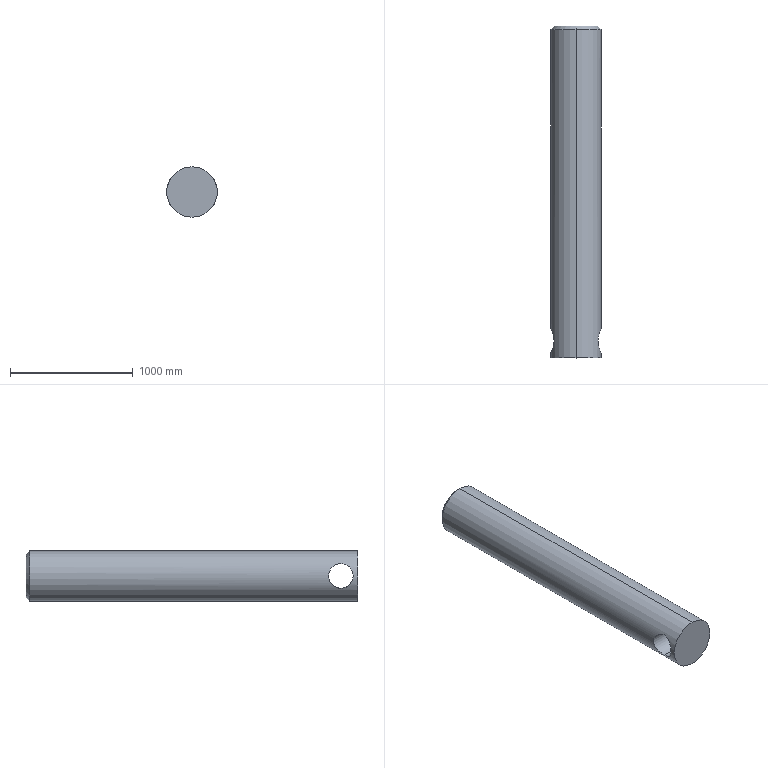Part | SolidWorks | features ICE 2, Chamfer 1, Extrusion 1 | 1 solid | 11 faces | box 410 x 2700 x 410 mm | volume 230530673 mm3 | cylinder 6 | plane 3 | cone 2 | commonest cylinder face diameters 200 x2 250 x2 410 x2
STEP:
#1=CARTESIAN_POINT('',(0.,2300.,175.));
#2=VERTEX_POINT('',#1);
#3=CARTESIAN_POINT('',(0.,2300.,-175.));
#4=VERTEX_POINT('',#3);
#5=CARTESIAN_POINT('',(0.,2300.,0.));
#6=DIRECTION('',(0.,1.,0.));
#7=DIRECTION('',(0.,0.,1.));
#8=AXIS2_PLACEMENT_3D('',#5,#6,#7);
#9=CIRCLE('',#8,175.);
#10=EDGE_CURVE('',#2,#4,#9,.T.);
#11=ORIENTED_EDGE('',*,*,#10,.F.);
#12=CARTESIAN_POINT('',(0.,2270.,205.));
#13=VERTEX_POINT('',#12);
#14=CARTESIAN_POINT('',(0.,2300.,175.));
#15=DIRECTION('',(0.,-0.7071,0.7071));
#16=VECTOR('',#15,1000.);
#17=LINE('',#14,#16);
#18=EDGE_CURVE('',#2,#13,#17,.T.);
#19=ORIENTED_EDGE('',*,*,#18,.T.);
#20=CARTESIAN_POINT('',(0.,2270.,-205.));
#21=VERTEX_POINT('',#20);
#22=CARTESIAN_POINT('',(0.,2270.,0.));
#23=DIRECTION('',(0.,-1.,0.));
#24=DIRECTION('',(0.,0.,1.));
#25=AXIS2_PLACEMENT_3D('',#22,#23,#24);
#26=CIRCLE('',#25,205.);
#27=EDGE_CURVE('',#21,#13,#26,.T.);
#28=ORIENTED_EDGE('',*,*,#27,.F.);
#29=CARTESIAN_POINT('',(0.,2300.,-175.));
#30=DIRECTION('',(0.,-0.7071,-0.7071));
#31=VECTOR('',#30,1000.);
#32=LINE('',#29,#31);
#33=EDGE_CURVE('',#4,#21,#32,.T.);
#34=ORIENTED_EDGE('',*,*,#33,.F.);
#35=EDGE_LOOP('',(#11,#19,#28,#34));
#36=FACE_OUTER_BOUND('',#35,.T.);
#37=CARTESIAN_POINT('',(0.,2300.,0.));
#38=DIRECTION('',(0.,-1.,0.));
#39=DIRECTION('',(0.,0.,-1.));
#40=AXIS2_PLACEMENT_3D('',#37,#38,#39);
#41=CONICAL_SURFACE('',#40,175.,0.7854);
#42=ADVANCED_FACE('',(#36),#41,.T.);
#43=CARTESIAN_POINT('',(178.955,-260.844,100.));
#44=VERTEX_POINT('',#43);
#45=CARTESIAN_POINT('',(178.955,-260.844,-100.));
#46=VERTEX_POINT('',#45);
#47=CARTESIAN_POINT('',(178.955,-260.844,100.));
#48=CARTESIAN_POINT('',(178.955,-264.207,100.));
#49=CARTESIAN_POINT('',(179.05,-267.535,99.831));
#50=CARTESIAN_POINT('',(179.417,-274.125,99.169));
#51=CARTESIAN_POINT('',(179.69,-277.387,98.677));
#52=CARTESIAN_POINT('',(180.399,-283.847,97.374));
#53=CARTESIAN_POINT('',(180.836,-287.044,96.563));
#54=CARTESIAN_POINT('',(181.477,-291.002,95.348));
#55=CARTESIAN_POINT('',(181.61,-291.792,95.094));
#56=CARTESIAN_POINT('',(181.884,-293.361,94.569));
#57=CARTESIAN_POINT('',(182.025,-294.141,94.297));
#58=CARTESIAN_POINT('',(182.459,-296.462,93.456));
#59=CARTESIAN_POINT('',(182.764,-297.988,92.86));
#60=CARTESIAN_POINT('',(183.717,-302.505,90.967));
#61=CARTESIAN_POINT('',(184.406,-305.433,89.567));
#62=CARTESIAN_POINT('',(185.867,-311.134,86.495));
#63=CARTESIAN_POINT('',(186.639,-313.906,84.823));
#64=CARTESIAN_POINT('',(187.841,-317.949,82.108));
#65=CARTESIAN_POINT('',(188.251,-319.28,81.165));
#66=CARTESIAN_POINT('',(189.074,-321.881,79.228));
#67=CARTESIAN_POINT('',(189.489,-323.153,78.231));
#68=CARTESIAN_POINT('',(190.738,-326.886,75.159));
#69=CARTESIAN_POINT('',(191.577,-329.263,73.001));
#70=CARTESIAN_POINT('',(193.244,-333.801,68.465));
#71=CARTESIAN_POINT('',(194.073,-335.963,66.087));
#72=CARTESIAN_POINT('',(195.293,-339.044,62.349));
#73=CARTESIAN_POINT('',(195.696,-340.043,61.074));
#74=CARTESIAN_POINT('',(196.292,-341.502,59.118));
#75=CARTESIAN_POINT('',(196.49,-341.982,58.457));
#76=CARTESIAN_POINT('',(196.881,-342.924,57.127));
#77=CARTESIAN_POINT('',(197.074,-343.386,56.457));
#78=CARTESIAN_POINT('',(198.028,-345.653,53.084));
#79=CARTESIAN_POINT('',(198.752,-347.327,50.31));
#80=CARTESIAN_POINT('',(200.109,-350.4,44.611));
#81=CARTESIAN_POINT('',(200.74,-351.8,41.685));
#82=CARTESIAN_POINT('',(201.895,-354.32,35.677));
#83=CARTESIAN_POINT('',(202.418,-355.441,32.594));
#84=CARTESIAN_POINT('',(203.107,-356.903,27.844));
#85=CARTESIAN_POINT('',(203.321,-357.355,26.235));
#86=CARTESIAN_POINT('',(203.711,-358.174,23.013));
#87=CARTESIAN_POINT('',(203.887,-358.542,21.397));
#88=CARTESIAN_POINT('',(204.358,-359.523,16.532));
#89=CARTESIAN_POINT('',(204.597,-360.015,13.268));
#90=CARTESIAN_POINT('',(204.917,-360.674,6.697));
#91=CARTESIAN_POINT('',(204.999,-360.842,3.391));
#92=CARTESIAN_POINT('',(205.001,-360.845,-1.601));
#93=CARTESIAN_POINT('',(204.981,-360.804,-3.27));
#94=CARTESIAN_POINT('',(204.92,-360.68,-5.782));
#95=CARTESIAN_POINT('',(204.895,-360.628,-6.622));
#96=CARTESIAN_POINT('',(204.834,-360.503,-8.294));
#97=CARTESIAN_POINT('',(204.798,-360.43,-9.127));
#98=CARTESIAN_POINT('',(204.596,-360.014,-13.279));
#99=CARTESIAN_POINT('',(204.356,-359.519,-16.557));
#100=CARTESIAN_POINT('',(203.728,-358.212,-23.029));
#101=CARTESIAN_POINT('',(203.341,-357.4,-26.224));
#102=CARTESIAN_POINT('',(202.656,-355.947,-30.953));
#103=CARTESIAN_POINT('',(202.411,-355.423,-32.519));
#104=CARTESIAN_POINT('',(201.886,-354.296,-35.63));
#105=CARTESIAN_POINT('',(201.607,-353.691,-37.176));
#106=CARTESIAN_POINT('',(200.731,-351.779,-41.733));
#107=CARTESIAN_POINT('',(200.094,-350.367,-44.679));
#108=CARTESIAN_POINT('',(198.73,-347.277,-50.397));
#109=CARTESIAN_POINT('',(198.004,-345.599,-53.17));
#110=CARTESIAN_POINT('',(196.862,-342.883,-57.202));
#111=CARTESIAN_POINT('',(196.473,-341.945,-58.525));
#112=CARTESIAN_POINT('',(195.678,-340.001,-61.129));
#113=CARTESIAN_POINT('',(195.273,-338.993,-62.413));
#114=CARTESIAN_POINT('',(194.045,-335.892,-66.169));
#115=CARTESIAN_POINT('',(193.213,-333.719,-68.553));
#116=CARTESIAN_POINT('',(191.543,-329.169,-73.089));
#117=CARTESIAN_POINT('',(190.705,-326.791,-75.242));
#118=CARTESIAN_POINT('',(189.045,-321.823,-79.321));
#119=CARTESIAN_POINT('',(188.223,-319.234,-81.248));
#120=CARTESIAN_POINT('',(187.019,-315.183,-83.964));
#121=CARTESIAN_POINT('',(186.622,-313.803,-84.841));
#122=CARTESIAN_POINT('',(185.851,-311.017,-86.518));
#123=CARTESIAN_POINT('',(185.475,-309.606,-87.32));
#124=CARTESIAN_POINT('',(184.38,-305.324,-89.621));
#125=CARTESIAN_POINT('',(183.694,-302.402,-91.014));
#126=CARTESIAN_POINT('',(182.433,-296.416,-93.516));
#127=CARTESIAN_POINT('',(181.858,-293.352,-94.625));
#128=CARTESIAN_POINT('',(181.095,-288.645,-96.072));
#129=CARTESIAN_POINT('',(180.858,-287.058,-96.517));
#130=CARTESIAN_POINT('',(180.53,-284.647,-97.129));
#131=CARTESIAN_POINT('',(180.425,-283.839,-97.324));
#132=CARTESIAN_POINT('',(180.225,-282.212,-97.694));
#133=CARTESIAN_POINT('',(180.13,-281.395,-97.869));
#134=CARTESIAN_POINT('',(179.682,-277.312,-98.691));
#135=CARTESIAN_POINT('',(179.411,-274.034,-99.181));
#136=CARTESIAN_POINT('',(179.047,-267.456,-99.836));
#137=CARTESIAN_POINT('',(178.955,-264.156,-100.));
#138=CARTESIAN_POINT('',(178.955,-260.844,-100.));
#139=B_SPLINE_CURVE_WITH_KNOTS('',3,(#47,#48,#49,#50,#51,#52,#53,#54,#55,#56,#57,#58,#59,#60,#61,#62,#63,#64,#65,#66,#67,#68,#69,#70,#71,#72,#73,#74,#75,#76,#77,#78,#79,#80,#81,#82,#83,#84,#85,#86,#87,#88,#89,#90,#91,#92,#93,#94,#95,#96,#97,#98,#99,#100,#101,#102,#103,#104,#105,#106,#107,#108,#109,#110,#111,#112,#113,#114,#115,#116,#117,#118,#119,#120,#121,#122,#123,#124,#125,#126,#127,#128,#129,#130,#131,#132,#133,#134,#135,#136,#137,#138),.UNSPECIFIED.,.F.,.F.,(4,2,2,2,2,2,2,2,2,2,2,2,2,2,2,2,2,2,2,2,2,2,2,2,2,2,2,2,2,2,2,2,2,2,2,2,2,2,2,2,2,2,2,2,2,4),(0.,0.00993,0.01986,0.02979,0.03227,0.03476,0.03972,0.04965,0.05958,0.06455,0.06951,0.07944,0.08937,0.09434,0.09682,0.0993,0.1092,0.1192,0.1291,0.1341,0.139,0.149,0.1589,0.1639,0.1663,0.1688,0.1787,0.1887,0.1936,0.1986,0.2085,0.2185,0.2234,0.2284,0.2383,0.2483,0.2582,0.2632,0.2681,0.278,0.288,0.2929,0.2954,0.2979,0.3078,0.3178),.UNSPECIFIED.);
#140=EDGE_CURVE('',#44,#46,#139,.T.);
#141=ORIENTED_EDGE('',*,*,#140,.T.);
#142=CARTESIAN_POINT('',(-178.955,-260.844,-100.));
#143=VERTEX_POINT('',#142);
#144=CARTESIAN_POINT('',(5000.,-260.844,-100.));
#145=DIRECTION('',(-1.,0.,0.));
#146=VECTOR('',#145,1000.);
#147=LINE('',#144,#146);
#148=EDGE_CURVE('',#46,#143,#147,.T.);
#149=ORIENTED_EDGE('',*,*,#148,.T.);
#150=CARTESIAN_POINT('',(-178.955,-260.844,100.));
#151=VERTEX_POINT('',#150);
#152=CARTESIAN_POINT('',(-178.955,-260.844,-100.));
#153=CARTESIAN_POINT('',(-178.955,-264.15,-100.));
#154=CARTESIAN_POINT('',(-179.047,-267.468,-99.836));
#155=CARTESIAN_POINT('',(-179.278,-271.63,-99.42));
#156=CARTESIAN_POINT('',(-179.33,-272.464,-99.326));
#157=CARTESIAN_POINT('',(-179.445,-274.123,-99.118));
#158=CARTESIAN_POINT('',(-179.509,-274.95,-99.004));
#159=CARTESIAN_POINT('',(-179.714,-277.418,-98.631));
#160=CARTESIAN_POINT('',(-179.872,-279.05,-98.343));
#161=CARTESIAN_POINT('',(-180.407,-283.906,-97.36));
#162=CARTESIAN_POINT('',(-180.843,-287.091,-96.55));
#163=CARTESIAN_POINT('',(-181.859,-293.36,-94.623));
#164=CARTESIAN_POINT('',(-182.438,-296.444,-93.506));
#165=CARTESIAN_POINT('',(-183.238,-300.237,-91.918));
#166=CARTESIAN_POINT('',(-183.402,-300.993,-91.59));
#167=CARTESIAN_POINT('',(-183.736,-302.491,-90.919));
#168=CARTESIAN_POINT('',(-183.906,-303.233,-90.575));
#169=CARTESIAN_POINT('',(-184.424,-305.444,-89.518));
#170=CARTESIAN_POINT('',(-184.78,-306.894,-88.781));
#171=CARTESIAN_POINT('',(-185.878,-311.175,-86.471));
#172=CARTESIAN_POINT('',(-186.648,-313.937,-84.802));
#173=CARTESIAN_POINT('',(-188.24,-319.288,-81.208));
#174=CARTESIAN_POINT('',(-189.062,-321.875,-79.282));
#175=CARTESIAN_POINT('',(-190.317,-325.627,-76.195));
#176=CARTESIAN_POINT('',(-190.74,-326.858,-75.132));
#177=CARTESIAN_POINT('',(-191.581,-329.252,-72.959));
#178=CARTESIAN_POINT('',(-192.001,-330.418,-71.847));
#179=CARTESIAN_POINT('',(-193.255,-333.83,-68.435));
#180=CARTESIAN_POINT('',(-194.082,-335.986,-66.06));
#181=CARTESIAN_POINT('',(-195.698,-340.067,-61.106));
#182=CARTESIAN_POINT('',(-196.488,-341.992,-58.527));
#183=CARTESIAN_POINT('',(-197.628,-344.704,-54.498));
#184=CARTESIAN_POINT('',(-198.001,-345.579,-53.129));
#185=CARTESIAN_POINT('',(-198.73,-347.268,-50.334));
#186=CARTESIAN_POINT('',(-199.086,-348.083,-48.908));
#187=CARTESIAN_POINT('',(-200.113,-350.411,-44.592));
#188=CARTESIAN_POINT('',(-200.747,-351.814,-41.652));
#189=CARTESIAN_POINT('',(-201.9,-354.33,-35.649));
#190=CARTESIAN_POINT('',(-202.418,-355.443,-32.585));
#191=CARTESIAN_POINT('',(-203.327,-357.371,-26.328));
#192=CARTESIAN_POINT('',(-203.717,-358.187,-23.136));
#193=CARTESIAN_POINT('',(-204.193,-359.179,-18.245));
#194=CARTESIAN_POINT('',(-204.334,-359.472,-16.592));
#195=CARTESIAN_POINT('',(-204.575,-359.971,-13.291));
#196=CARTESIAN_POINT('',(-204.676,-360.178,-11.64));
#197=CARTESIAN_POINT('',(-204.918,-360.675,-6.686));
#198=CARTESIAN_POINT('',(-204.999,-360.841,-3.381));
#199=CARTESIAN_POINT('',(-205.001,-360.846,3.232));
#200=CARTESIAN_POINT('',(-204.922,-360.685,6.541));
#201=CARTESIAN_POINT('',(-204.683,-360.193,11.507));
#202=CARTESIAN_POINT('',(-204.584,-359.988,13.163));
#203=CARTESIAN_POINT('',(-204.344,-359.491,16.476));
#204=CARTESIAN_POINT('',(-204.204,-359.202,18.121));
#205=CARTESIAN_POINT('',(-203.731,-358.218,23.006));
#206=CARTESIAN_POINT('',(-203.343,-357.406,26.203));
#207=CARTESIAN_POINT('',(-202.435,-355.478,32.483));
#208=CARTESIAN_POINT('',(-201.915,-354.363,35.567));
#209=CARTESIAN_POINT('',(-201.044,-352.463,40.108));
#210=CARTESIAN_POINT('',(-200.739,-351.792,41.607));
#211=CARTESIAN_POINT('',(-200.26,-350.728,43.836));
#212=CARTESIAN_POINT('',(-200.097,-350.363,44.575));
#213=CARTESIAN_POINT('',(-199.765,-349.62,46.038));
#214=CARTESIAN_POINT('',(-199.596,-349.24,46.764));
#215=CARTESIAN_POINT('',(-198.74,-347.3,50.359));
#216=CARTESIAN_POINT('',(-198.014,-345.621,53.134));
#217=CARTESIAN_POINT('',(-196.497,-342.015,58.495));
#218=CARTESIAN_POINT('',(-195.707,-340.088,61.079));
#219=CARTESIAN_POINT('',(-194.488,-337.011,64.816));
#220=CARTESIAN_POINT('',(-194.076,-335.954,66.039));
#221=CARTESIAN_POINT('',(-193.243,-333.776,68.437));
#222=CARTESIAN_POINT('',(-192.822,-332.652,69.614));
#223=CARTESIAN_POINT('',(-191.56,-329.217,73.045));
#224=CARTESIAN_POINT('',(-190.72,-326.832,75.206));
#225=CARTESIAN_POINT('',(-189.061,-321.873,79.282));
#226=CARTESIAN_POINT('',(-188.244,-319.3,81.199));
#227=CARTESIAN_POINT('',(-186.654,-313.959,84.789));
#228=CARTESIAN_POINT('',(-185.882,-311.191,86.463));
#229=CARTESIAN_POINT('',(-184.777,-306.883,88.786));
#230=CARTESIAN_POINT('',(-184.417,-305.418,89.531));
#231=CARTESIAN_POINT('',(-183.726,-302.466,90.941));
#232=CARTESIAN_POINT('',(-183.394,-300.977,91.608));
#233=CARTESIAN_POINT('',(-182.443,-296.467,93.496));
#234=CARTESIAN_POINT('',(-181.868,-293.407,94.606));
#235=CARTESIAN_POINT('',(-180.856,-287.173,96.527));
#236=CARTESIAN_POINT('',(-180.419,-284.,97.338));
#237=CARTESIAN_POINT('',(-179.882,-279.152,98.323));
#238=CARTESIAN_POINT('',(-179.723,-277.522,98.613));
#239=CARTESIAN_POINT('',(-179.517,-275.053,98.989));
#240=CARTESIAN_POINT('',(-179.453,-274.226,99.104));
#241=CARTESIAN_POINT('',(-179.337,-272.564,99.314));
#242=CARTESIAN_POINT('',(-179.284,-271.73,99.409));
#243=CARTESIAN_POINT('',(-179.144,-269.227,99.662));
#244=CARTESIAN_POINT('',(-179.073,-267.555,99.789));
#245=CARTESIAN_POINT('',(-179.003,-265.042,99.915));
#246=CARTESIAN_POINT('',(-178.985,-264.203,99.947));
#247=CARTESIAN_POINT('',(-178.961,-262.525,99.989));
#248=CARTESIAN_POINT('',(-178.955,-261.683,100.));
#249=CARTESIAN_POINT('',(-178.955,-260.844,100.));
#250=B_SPLINE_CURVE_WITH_KNOTS('',3,(#152,#153,#154,#155,#156,#157,#158,#159,#160,#161,#162,#163,#164,#165,#166,#167,#168,#169,#170,#171,#172,#173,#174,#175,#176,#177,#178,#179,#180,#181,#182,#183,#184,#185,#186,#187,#188,#189,#190,#191,#192,#193,#194,#195,#196,#197,#198,#199,#200,#201,#202,#203,#204,#205,#206,#207,#208,#209,#210,#211,#212,#213,#214,#215,#216,#217,#218,#219,#220,#221,#222,#223,#224,#225,#226,#227,#228,#229,#230,#231,#232,#233,#234,#235,#236,#237,#238,#239,#240,#241,#242,#243,#244,#245,#246,#247,#248,#249),.UNSPECIFIED.,.F.,.F.,(4,2,2,2,2,2,2,2,2,2,2,2,2,2,2,2,2,2,2,2,2,2,2,2,2,2,2,2,2,2,2,2,2,2,2,2,2,2,2,2,2,2,2,2,2,2,2,2,4),(0.3178,0.3277,0.3302,0.3326,0.3376,0.3475,0.3574,0.3599,0.3624,0.3673,0.3773,0.3872,0.3921,0.3971,0.407,0.4169,0.4219,0.4268,0.4367,0.4467,0.4566,0.4615,0.4665,0.4764,0.4863,0.4913,0.4962,0.5061,0.5161,0.521,0.5235,0.526,0.5359,0.5458,0.5508,0.5557,0.5656,0.5755,0.5855,0.5904,0.5954,0.6053,0.6152,0.6202,0.6226,0.6251,0.6301,0.6326,0.635),.UNSPECIFIED.);
#251=EDGE_CURVE('',#143,#151,#250,.T.);
#252=ORIENTED_EDGE('',*,*,#251,.T.);
#253=CARTESIAN_POINT('',(5000.,-260.844,100.));
#254=DIRECTION('',(-1.,0.,0.));
#255=VECTOR('',#254,1000.);
#256=LINE('',#253,#255);
#257=EDGE_CURVE('',#44,#151,#256,.T.);
#258=ORIENTED_EDGE('',*,*,#257,.F.);
#259=EDGE_LOOP('',(#141,#149,#252,#258));
#260=FACE_OUTER_BOUND('',#259,.T.);
#261=CARTESIAN_POINT('',(5000.,-260.844,0.));
#262=DIRECTION('',(-1.,0.,0.));
#263=DIRECTION('',(0.,0.,1.));
#264=AXIS2_PLACEMENT_3D('',#261,#262,#263);
#265=CYLINDRICAL_SURFACE('',#264,100.);
#266=ADVANCED_FACE('',(#260),#265,.F.);
#267=CARTESIAN_POINT('',(0.,2300.,-125.));
#268=VERTEX_POINT('',#267);
#269=CARTESIAN_POINT('',(0.,2300.,125.));
#270=VERTEX_POINT('',#269);
#271=CARTESIAN_POINT('',(0.,2300.,0.));
#272=DIRECTION('',(0.,1.,0.));
#273=DIRECTION('',(0.,0.,1.));
#274=AXIS2_PLACEMENT_3D('',#271,#272,#273);
#275=CIRCLE('',#274,125.);
#276=EDGE_CURVE('',#268,#270,#275,.T.);
#277=ORIENTED_EDGE('',*,*,#276,.T.);
#278=CARTESIAN_POINT('',(0.,0.,125.));
#279=VERTEX_POINT('',#278);
#280=CARTESIAN_POINT('',(0.,2300.,125.));
#281=DIRECTION('',(0.,-1.,0.));
#282=VECTOR('',#281,1000.);
#283=LINE('',#280,#282);
#284=EDGE_CURVE('',#270,#279,#283,.T.);
#285=ORIENTED_EDGE('',*,*,#284,.T.);
#286=CARTESIAN_POINT('',(0.,0.,-125.));
#287=VERTEX_POINT('',#286);
#288=CARTESIAN_POINT('',(0.,0.,0.));
#289=DIRECTION('',(0.,1.,0.));
#290=DIRECTION('',(0.,0.,1.));
#291=AXIS2_PLACEMENT_3D('',#288,#289,#290);
#292=CIRCLE('',#291,125.);
#293=EDGE_CURVE('',#287,#279,#292,.T.);
#294=ORIENTED_EDGE('',*,*,#293,.F.);
#295=CARTESIAN_POINT('',(0.,2300.,-125.));
#296=DIRECTION('',(0.,-1.,0.));
#297=VECTOR('',#296,1000.);
#298=LINE('',#295,#297);
#299=EDGE_CURVE('',#268,#287,#298,.T.);
#300=ORIENTED_EDGE('',*,*,#299,.F.);
#301=EDGE_LOOP('',(#277,#285,#294,#300));
#302=FACE_OUTER_BOUND('',#301,.T.);
#303=CARTESIAN_POINT('',(0.,2300.,0.));
#304=DIRECTION('',(0.,-1.,0.));
#305=DIRECTION('',(0.,0.,-1.));
#306=AXIS2_PLACEMENT_3D('',#303,#304,#305);
#307=CYLINDRICAL_SURFACE('',#306,125.);
#308=ADVANCED_FACE('',(#302),#307,.F.);
#309=ORIENTED_EDGE('',*,*,#140,.F.);
#310=CARTESIAN_POINT('',(178.955,-260.844,-100.));
#311=CARTESIAN_POINT('',(178.955,-257.537,-100.));
#312=CARTESIAN_POINT('',(179.047,-254.219,-99.836));
#313=CARTESIAN_POINT('',(179.278,-250.057,-99.42));
#314=CARTESIAN_POINT('',(179.33,-249.223,-99.326));
#315=CARTESIAN_POINT('',(179.445,-247.564,-99.118));
#316=CARTESIAN_POINT('',(179.509,-246.738,-99.004));
#317=CARTESIAN_POINT('',(179.714,-244.269,-98.631));
#318=CARTESIAN_POINT('',(179.872,-242.637,-98.343));
#319=CARTESIAN_POINT('',(180.407,-237.781,-97.36));
#320=CARTESIAN_POINT('',(180.843,-234.596,-96.55));
#321=CARTESIAN_POINT('',(181.859,-228.327,-94.623));
#322=CARTESIAN_POINT('',(182.438,-225.243,-93.506));
#323=CARTESIAN_POINT('',(183.238,-221.45,-91.918));
#324=CARTESIAN_POINT('',(183.402,-220.694,-91.59));
#325=CARTESIAN_POINT('',(183.736,-219.197,-90.919));
#326=CARTESIAN_POINT('',(183.906,-218.454,-90.575));
#327=CARTESIAN_POINT('',(184.424,-216.244,-89.518));
#328=CARTESIAN_POINT('',(184.78,-214.794,-88.781));
#329=CARTESIAN_POINT('',(185.878,-210.513,-86.471));
#330=CARTESIAN_POINT('',(186.648,-207.75,-84.802));
#331=CARTESIAN_POINT('',(188.24,-202.4,-81.208));
#332=CARTESIAN_POINT('',(189.062,-199.812,-79.282));
#333=CARTESIAN_POINT('',(190.317,-196.06,-76.195));
#334=CARTESIAN_POINT('',(190.74,-194.83,-75.132));
#335=CARTESIAN_POINT('',(191.581,-192.436,-72.959));
#336=CARTESIAN_POINT('',(192.001,-191.269,-71.847));
#337=CARTESIAN_POINT('',(193.255,-187.858,-68.435));
#338=CARTESIAN_POINT('',(194.082,-185.701,-66.06));
#339=CARTESIAN_POINT('',(195.698,-181.62,-61.106));
#340=CARTESIAN_POINT('',(196.488,-179.695,-58.527));
#341=CARTESIAN_POINT('',(197.628,-176.983,-54.498));
#342=CARTESIAN_POINT('',(198.001,-176.109,-53.129));
#343=CARTESIAN_POINT('',(198.73,-174.42,-50.334));
#344=CARTESIAN_POINT('',(199.086,-173.604,-48.908));
#345=CARTESIAN_POINT('',(200.113,-171.277,-44.592));
#346=CARTESIAN_POINT('',(200.747,-169.873,-41.652));
#347=CARTESIAN_POINT('',(201.9,-167.357,-35.649));
#348=CARTESIAN_POINT('',(202.418,-166.245,-32.585));
#349=CARTESIAN_POINT('',(203.327,-164.316,-26.328));
#350=CARTESIAN_POINT('',(203.717,-163.5,-23.136));
#351=CARTESIAN_POINT('',(204.193,-162.508,-18.245));
#352=CARTESIAN_POINT('',(204.334,-162.216,-16.592));
#353=CARTESIAN_POINT('',(204.575,-161.717,-13.291));
#354=CARTESIAN_POINT('',(204.676,-161.51,-11.64));
#355=CARTESIAN_POINT('',(204.918,-161.012,-6.686));
#356=CARTESIAN_POINT('',(204.999,-160.846,-3.381));
#357=CARTESIAN_POINT('',(205.001,-160.841,3.232));
#358=CARTESIAN_POINT('',(204.922,-161.002,6.541));
#359=CARTESIAN_POINT('',(204.683,-161.494,11.507));
#360=CARTESIAN_POINT('',(204.584,-161.7,13.163));
#361=CARTESIAN_POINT('',(204.344,-162.196,16.476));
#362=CARTESIAN_POINT('',(204.204,-162.485,18.121));
#363=CARTESIAN_POINT('',(203.731,-163.469,23.006));
#364=CARTESIAN_POINT('',(203.343,-164.282,26.203));
#365=CARTESIAN_POINT('',(202.435,-166.21,32.483));
#366=CARTESIAN_POINT('',(201.915,-167.325,35.567));
#367=CARTESIAN_POINT('',(201.044,-169.225,40.108));
#368=CARTESIAN_POINT('',(200.739,-169.896,41.607));
#369=CARTESIAN_POINT('',(200.26,-170.96,43.836));
#370=CARTESIAN_POINT('',(200.097,-171.324,44.575));
#371=CARTESIAN_POINT('',(199.765,-172.068,46.038));
#372=CARTESIAN_POINT('',(199.596,-172.448,46.764));
#373=CARTESIAN_POINT('',(198.74,-174.387,50.359));
#374=CARTESIAN_POINT('',(198.014,-176.066,53.134));
#375=CARTESIAN_POINT('',(196.497,-179.672,58.495));
#376=CARTESIAN_POINT('',(195.707,-181.599,61.079));
#377=CARTESIAN_POINT('',(194.488,-184.677,64.816));
#378=CARTESIAN_POINT('',(194.076,-185.734,66.039));
#379=CARTESIAN_POINT('',(193.243,-187.912,68.437));
#380=CARTESIAN_POINT('',(192.822,-189.035,69.614));
#381=CARTESIAN_POINT('',(191.56,-192.471,73.045));
#382=CARTESIAN_POINT('',(190.72,-194.856,75.206));
#383=CARTESIAN_POINT('',(189.061,-199.814,79.282));
#384=CARTESIAN_POINT('',(188.244,-202.388,81.199));
#385=CARTESIAN_POINT('',(186.654,-207.729,84.789));
#386=CARTESIAN_POINT('',(185.882,-210.497,86.463));
#387=CARTESIAN_POINT('',(184.777,-214.804,88.786));
#388=CARTESIAN_POINT('',(184.417,-216.27,89.531));
#389=CARTESIAN_POINT('',(183.726,-219.221,90.941));
#390=CARTESIAN_POINT('',(183.394,-220.711,91.608));
#391=CARTESIAN_POINT('',(182.443,-225.22,93.496));
#392=CARTESIAN_POINT('',(181.868,-228.281,94.606));
#393=CARTESIAN_POINT('',(180.856,-234.514,96.527));
#394=CARTESIAN_POINT('',(180.419,-237.687,97.338));
#395=CARTESIAN_POINT('',(179.882,-242.535,98.323));
#396=CARTESIAN_POINT('',(179.723,-244.166,98.613));
#397=CARTESIAN_POINT('',(179.517,-246.635,98.989));
#398=CARTESIAN_POINT('',(179.453,-247.462,99.104));
#399=CARTESIAN_POINT('',(179.337,-249.123,99.314));
#400=CARTESIAN_POINT('',(179.284,-249.958,99.409));
#401=CARTESIAN_POINT('',(179.144,-252.461,99.662));
#402=CARTESIAN_POINT('',(179.073,-254.133,99.789));
#403=CARTESIAN_POINT('',(179.003,-256.646,99.915));
#404=CARTESIAN_POINT('',(178.985,-257.484,99.947));
#405=CARTESIAN_POINT('',(178.961,-259.163,99.989));
#406=CARTESIAN_POINT('',(178.955,-260.004,100.));
#407=CARTESIAN_POINT('',(178.955,-260.844,100.));
#408=B_SPLINE_CURVE_WITH_KNOTS('',3,(#310,#311,#312,#313,#314,#315,#316,#317,#318,#319,#320,#321,#322,#323,#324,#325,#326,#327,#328,#329,#330,#331,#332,#333,#334,#335,#336,#337,#338,#339,#340,#341,#342,#343,#344,#345,#346,#347,#348,#349,#350,#351,#352,#353,#354,#355,#356,#357,#358,#359,#360,#361,#362,#363,#364,#365,#366,#367,#368,#369,#370,#371,#372,#373,#374,#375,#376,#377,#378,#379,#380,#381,#382,#383,#384,#385,#386,#387,#388,#389,#390,#391,#392,#393,#394,#395,#396,#397,#398,#399,#400,#401,#402,#403,#404,#405,#406,#407),.UNSPECIFIED.,.F.,.F.,(4,2,2,2,2,2,2,2,2,2,2,2,2,2,2,2,2,2,2,2,2,2,2,2,2,2,2,2,2,2,2,2,2,2,2,2,2,2,2,2,2,2,2,2,2,2,2,2,4),(0.3178,0.3277,0.3302,0.3326,0.3376,0.3475,0.3574,0.3599,0.3624,0.3673,0.3773,0.3872,0.3921,0.3971,0.407,0.4169,0.4219,0.4268,0.4367,0.4467,0.4566,0.4615,0.4665,0.4764,0.4863,0.4913,0.4962,0.5061,0.5161,0.521,0.5235,0.526,0.5359,0.5458,0.5508,0.5557,0.5656,0.5755,0.5855,0.5904,0.5954,0.6053,0.6152,0.6202,0.6226,0.6251,0.6301,0.6326,0.635),.UNSPECIFIED.);
#409=EDGE_CURVE('',#46,#44,#408,.T.);
#410=ORIENTED_EDGE('',*,*,#409,.F.);
#411=EDGE_LOOP('',(#309,#410));
#412=FACE_BOUND('',#411,.T.);
#413=ORIENTED_EDGE('',*,*,#27,.T.);
#414=CARTESIAN_POINT('',(0.,-400.,205.));
#415=VERTEX_POINT('',#414);
#416=CARTESIAN_POINT('',(0.,2300.,205.));
#417=DIRECTION('',(0.,-1.,0.));
#418=VECTOR('',#417,1000.);
#419=LINE('',#416,#418);
#420=EDGE_CURVE('',#13,#415,#419,.T.);
#421=ORIENTED_EDGE('',*,*,#420,.T.);
#422=CARTESIAN_POINT('',(0.,-400.,-205.));
#423=VERTEX_POINT('',#422);
#424=CARTESIAN_POINT('',(0.,-400.,0.));
#425=DIRECTION('',(0.,-1.,0.));
#426=DIRECTION('',(0.,0.,-1.));
#427=AXIS2_PLACEMENT_3D('',#424,#425,#426);
#428=CIRCLE('',#427,205.);
#429=EDGE_CURVE('',#423,#415,#428,.T.);
#430=ORIENTED_EDGE('',*,*,#429,.F.);
#431=CARTESIAN_POINT('',(0.,2300.,-205.));
#432=DIRECTION('',(0.,-1.,0.));
#433=VECTOR('',#432,1000.);
#434=LINE('',#431,#433);
#435=EDGE_CURVE('',#21,#423,#434,.T.);
#436=ORIENTED_EDGE('',*,*,#435,.F.);
#437=EDGE_LOOP('',(#413,#421,#430,#436));
#438=FACE_OUTER_BOUND('',#437,.T.);
#439=CARTESIAN_POINT('',(0.,2300.,0.));
#440=DIRECTION('',(0.,-1.,0.));
#441=DIRECTION('',(0.,0.,-1.));
#442=AXIS2_PLACEMENT_3D('',#439,#440,#441);
#443=CYLINDRICAL_SURFACE('',#442,205.);
#444=ADVANCED_FACE('',(#412,#438),#443,.T.);
#445=ORIENTED_EDGE('',*,*,#420,.F.);
#446=CARTESIAN_POINT('',(0.,2270.,0.));
#447=DIRECTION('',(0.,-1.,0.));
#448=DIRECTION('',(0.,0.,1.));
#449=AXIS2_PLACEMENT_3D('',#446,#447,#448);
#450=CIRCLE('',#449,205.);
#451=EDGE_CURVE('',#13,#21,#450,.T.);
#452=ORIENTED_EDGE('',*,*,#451,.T.);
#453=ORIENTED_EDGE('',*,*,#435,.T.);
#454=CARTESIAN_POINT('',(0.,-400.,0.));
#455=DIRECTION('',(0.,-1.,0.));
#456=DIRECTION('',(0.,0.,-1.));
#457=AXIS2_PLACEMENT_3D('',#454,#455,#456);
#458=CIRCLE('',#457,205.);
#459=EDGE_CURVE('',#415,#423,#458,.T.);
#460=ORIENTED_EDGE('',*,*,#459,.F.);
#461=EDGE_LOOP('',(#445,#452,#453,#460));
#462=FACE_OUTER_BOUND('',#461,.T.);
#463=CARTESIAN_POINT('',(-178.955,-260.844,100.));
#464=CARTESIAN_POINT('',(-178.955,-257.481,100.));
#465=CARTESIAN_POINT('',(-179.05,-254.153,99.831));
#466=CARTESIAN_POINT('',(-179.417,-247.562,99.169));
#467=CARTESIAN_POINT('',(-179.69,-244.3,98.677));
#468=CARTESIAN_POINT('',(-180.399,-237.841,97.374));
#469=CARTESIAN_POINT('',(-180.836,-234.643,96.563));
#470=CARTESIAN_POINT('',(-181.477,-230.686,95.348));
#471=CARTESIAN_POINT('',(-181.61,-229.895,95.094));
#472=CARTESIAN_POINT('',(-181.884,-228.326,94.569));
#473=CARTESIAN_POINT('',(-182.025,-227.547,94.297));
#474=CARTESIAN_POINT('',(-182.459,-225.226,93.456));
#475=CARTESIAN_POINT('',(-182.764,-223.699,92.86));
#476=CARTESIAN_POINT('',(-183.717,-219.183,90.967));
#477=CARTESIAN_POINT('',(-184.406,-216.254,89.567));
#478=CARTESIAN_POINT('',(-185.867,-210.554,86.495));
#479=CARTESIAN_POINT('',(-186.639,-207.781,84.823));
#480=CARTESIAN_POINT('',(-187.841,-203.739,82.108));
#481=CARTESIAN_POINT('',(-188.251,-202.407,81.165));
#482=CARTESIAN_POINT('',(-189.074,-199.806,79.228));
#483=CARTESIAN_POINT('',(-189.489,-198.534,78.231));
#484=CARTESIAN_POINT('',(-190.738,-194.802,75.159));
#485=CARTESIAN_POINT('',(-191.577,-192.425,73.001));
#486=CARTESIAN_POINT('',(-193.244,-187.886,68.465));
#487=CARTESIAN_POINT('',(-194.073,-185.724,66.087));
#488=CARTESIAN_POINT('',(-195.293,-182.644,62.349));
#489=CARTESIAN_POINT('',(-195.696,-181.644,61.074));
#490=CARTESIAN_POINT('',(-196.292,-180.185,59.118));
#491=CARTESIAN_POINT('',(-196.49,-179.706,58.457));
#492=CARTESIAN_POINT('',(-196.881,-178.764,57.127));
#493=CARTESIAN_POINT('',(-197.074,-178.301,56.457));
#494=CARTESIAN_POINT('',(-198.028,-176.034,53.084));
#495=CARTESIAN_POINT('',(-198.752,-174.36,50.31));
#496=CARTESIAN_POINT('',(-200.109,-171.287,44.611));
#497=CARTESIAN_POINT('',(-200.74,-169.888,41.685));
#498=CARTESIAN_POINT('',(-201.895,-167.368,35.677));
#499=CARTESIAN_POINT('',(-202.418,-166.247,32.594));
#500=CARTESIAN_POINT('',(-203.107,-164.784,27.844));
#501=CARTESIAN_POINT('',(-203.321,-164.332,26.235));
#502=CARTESIAN_POINT('',(-203.711,-163.514,23.013));
#503=CARTESIAN_POINT('',(-203.887,-163.146,21.397));
#504=CARTESIAN_POINT('',(-204.358,-162.164,16.532));
#505=CARTESIAN_POINT('',(-204.597,-161.673,13.268));
#506=CARTESIAN_POINT('',(-204.917,-161.014,6.697));
#507=CARTESIAN_POINT('',(-204.999,-160.846,3.391));
#508=CARTESIAN_POINT('',(-205.001,-160.843,-1.601));
#509=CARTESIAN_POINT('',(-204.981,-160.883,-3.27));
#510=CARTESIAN_POINT('',(-204.92,-161.008,-5.782));
#511=CARTESIAN_POINT('',(-204.895,-161.06,-6.622));
#512=CARTESIAN_POINT('',(-204.834,-161.185,-8.294));
#513=CARTESIAN_POINT('',(-204.798,-161.258,-9.127));
#514=CARTESIAN_POINT('',(-204.596,-161.673,-13.279));
#515=CARTESIAN_POINT('',(-204.356,-162.169,-16.557));
#516=CARTESIAN_POINT('',(-203.728,-163.476,-23.029));
#517=CARTESIAN_POINT('',(-203.341,-164.287,-26.224));
#518=CARTESIAN_POINT('',(-202.656,-165.74,-30.953));
#519=CARTESIAN_POINT('',(-202.411,-166.264,-32.519));
#520=CARTESIAN_POINT('',(-201.886,-167.392,-35.63));
#521=CARTESIAN_POINT('',(-201.607,-167.996,-37.176));
#522=CARTESIAN_POINT('',(-200.731,-169.908,-41.733));
#523=CARTESIAN_POINT('',(-200.094,-171.321,-44.679));
#524=CARTESIAN_POINT('',(-198.73,-174.411,-50.397));
#525=CARTESIAN_POINT('',(-198.004,-176.089,-53.17));
#526=CARTESIAN_POINT('',(-196.862,-178.804,-57.202));
#527=CARTESIAN_POINT('',(-196.473,-179.743,-58.525));
#528=CARTESIAN_POINT('',(-195.678,-181.687,-61.129));
#529=CARTESIAN_POINT('',(-195.273,-182.695,-62.413));
#530=CARTESIAN_POINT('',(-194.045,-185.796,-66.169));
#531=CARTESIAN_POINT('',(-193.213,-187.968,-68.553));
#532=CARTESIAN_POINT('',(-191.543,-192.519,-73.089));
#533=CARTESIAN_POINT('',(-190.705,-194.897,-75.242));
#534=CARTESIAN_POINT('',(-189.045,-199.865,-79.321));
#535=CARTESIAN_POINT('',(-188.223,-202.454,-81.248));
#536=CARTESIAN_POINT('',(-187.019,-206.505,-83.964));
#537=CARTESIAN_POINT('',(-186.622,-207.884,-84.841));
#538=CARTESIAN_POINT('',(-185.851,-210.671,-86.518));
#539=CARTESIAN_POINT('',(-185.475,-212.081,-87.32));
#540=CARTESIAN_POINT('',(-184.38,-216.363,-89.621));
#541=CARTESIAN_POINT('',(-183.694,-219.286,-91.014));
#542=CARTESIAN_POINT('',(-182.433,-225.272,-93.516));
#543=CARTESIAN_POINT('',(-181.858,-228.335,-94.625));
#544=CARTESIAN_POINT('',(-181.095,-233.042,-96.072));
#545=CARTESIAN_POINT('',(-180.858,-234.63,-96.517));
#546=CARTESIAN_POINT('',(-180.53,-237.04,-97.129));
#547=CARTESIAN_POINT('',(-180.425,-237.849,-97.324));
#548=CARTESIAN_POINT('',(-180.225,-239.475,-97.694));
#549=CARTESIAN_POINT('',(-180.13,-240.292,-97.869));
#550=CARTESIAN_POINT('',(-179.682,-244.375,-98.691));
#551=CARTESIAN_POINT('',(-179.411,-247.653,-99.181));
#552=CARTESIAN_POINT('',(-179.047,-254.232,-99.836));
#553=CARTESIAN_POINT('',(-178.955,-257.532,-100.));
#554=CARTESIAN_POINT('',(-178.955,-260.844,-100.));
#555=B_SPLINE_CURVE_WITH_KNOTS('',3,(#463,#464,#465,#466,#467,#468,#469,#470,#471,#472,#473,#474,#475,#476,#477,#478,#479,#480,#481,#482,#483,#484,#485,#486,#487,#488,#489,#490,#491,#492,#493,#494,#495,#496,#497,#498,#499,#500,#501,#502,#503,#504,#505,#506,#507,#508,#509,#510,#511,#512,#513,#514,#515,#516,#517,#518,#519,#520,#521,#522,#523,#524,#525,#526,#527,#528,#529,#530,#531,#532,#533,#534,#535,#536,#537,#538,#539,#540,#541,#542,#543,#544,#545,#546,#547,#548,#549,#550,#551,#552,#553,#554),.UNSPECIFIED.,.F.,.F.,(4,2,2,2,2,2,2,2,2,2,2,2,2,2,2,2,2,2,2,2,2,2,2,2,2,2,2,2,2,2,2,2,2,2,2,2,2,2,2,2,2,2,2,2,2,4),(0.,0.00993,0.01986,0.02979,0.03227,0.03476,0.03972,0.04965,0.05958,0.06455,0.06951,0.07944,0.08937,0.09434,0.09682,0.0993,0.1092,0.1192,0.1291,0.1341,0.139,0.149,0.1589,0.1639,0.1663,0.1688,0.1787,0.1887,0.1936,0.1986,0.2085,0.2185,0.2234,0.2284,0.2383,0.2483,0.2582,0.2632,0.2681,0.278,0.288,0.2929,0.2954,0.2979,0.3078,0.3178),.UNSPECIFIED.);
#556=EDGE_CURVE('',#151,#143,#555,.T.);
#557=ORIENTED_EDGE('',*,*,#556,.F.);
#558=ORIENTED_EDGE('',*,*,#251,.F.);
#559=EDGE_LOOP('',(#557,#558));
#560=FACE_BOUND('',#559,.T.);
#561=CARTESIAN_POINT('',(0.,2300.,0.));
#562=DIRECTION('',(0.,-1.,0.));
#563=DIRECTION('',(0.,0.,-1.));
#564=AXIS2_PLACEMENT_3D('',#561,#562,#563);
#565=CYLINDRICAL_SURFACE('',#564,205.);
#566=ADVANCED_FACE('',(#462,#560),#565,.T.);
#567=CARTESIAN_POINT('',(0.,2300.,0.));
#568=DIRECTION('',(0.,1.,0.));
#569=DIRECTION('',(0.,0.,1.));
#570=AXIS2_PLACEMENT_3D('',#567,#568,#569);
#571=CIRCLE('',#570,175.);
#572=EDGE_CURVE('',#4,#2,#571,.T.);
#573=ORIENTED_EDGE('',*,*,#572,.T.);
#574=ORIENTED_EDGE('',*,*,#10,.T.);
#575=EDGE_LOOP('',(#573,#574));
#576=FACE_OUTER_BOUND('',#575,.T.);
#577=ORIENTED_EDGE('',*,*,#276,.F.);
#578=CARTESIAN_POINT('',(0.,2300.,0.));
#579=DIRECTION('',(0.,1.,0.));
#580=DIRECTION('',(0.,0.,1.));
#581=AXIS2_PLACEMENT_3D('',#578,#579,#580);
#582=CIRCLE('',#581,125.);
#583=EDGE_CURVE('',#270,#268,#582,.T.);
#584=ORIENTED_EDGE('',*,*,#583,.F.);
#585=EDGE_LOOP('',(#577,#584));
#586=FACE_BOUND('',#585,.T.);
#587=CARTESIAN_POINT('',(0.,2300.,0.));
#588=DIRECTION('',(0.,1.,0.));
#589=DIRECTION('',(0.,0.,1.));
#590=AXIS2_PLACEMENT_3D('',#587,#588,#589);
#591=PLANE('',#590);
#592=ADVANCED_FACE('',(#576,#586),#591,.T.);
#593=ORIENTED_EDGE('',*,*,#284,.F.);
#594=ORIENTED_EDGE('',*,*,#583,.T.);
#595=ORIENTED_EDGE('',*,*,#299,.T.);
#596=CARTESIAN_POINT('',(0.,0.,0.));
#597=DIRECTION('',(0.,1.,0.));
#598=DIRECTION('',(0.,0.,1.));
#599=AXIS2_PLACEMENT_3D('',#596,#597,#598);
#600=CIRCLE('',#599,125.);
#601=EDGE_CURVE('',#279,#287,#600,.T.);
#602=ORIENTED_EDGE('',*,*,#601,.F.);
#603=EDGE_LOOP('',(#593,#594,#595,#602));
#604=FACE_OUTER_BOUND('',#603,.T.);
#605=CARTESIAN_POINT('',(0.,2300.,0.));
#606=DIRECTION('',(0.,-1.,0.));
#607=DIRECTION('',(0.,0.,-1.));
#608=AXIS2_PLACEMENT_3D('',#605,#606,#607);
#609=CYLINDRICAL_SURFACE('',#608,125.);
#610=ADVANCED_FACE('',(#604),#609,.F.);
#611=ORIENTED_EDGE('',*,*,#293,.T.);
#612=ORIENTED_EDGE('',*,*,#601,.T.);
#613=EDGE_LOOP('',(#611,#612));
#614=FACE_OUTER_BOUND('',#613,.T.);
#615=CARTESIAN_POINT('',(0.,0.,0.));
#616=DIRECTION('',(0.,-1.,0.));
#617=DIRECTION('',(0.,0.,-1.));
#618=AXIS2_PLACEMENT_3D('',#615,#616,#617);
#619=PLANE('',#618);
#620=ADVANCED_FACE('',(#614),#619,.F.);
#621=ORIENTED_EDGE('',*,*,#429,.T.);
#622=ORIENTED_EDGE('',*,*,#459,.T.);
#623=EDGE_LOOP('',(#621,#622));
#624=FACE_OUTER_BOUND('',#623,.T.);
#625=CARTESIAN_POINT('',(0.,-400.,0.));
#626=DIRECTION('',(0.,-1.,0.));
#627=DIRECTION('',(0.,0.,-1.));
#628=AXIS2_PLACEMENT_3D('',#625,#626,#627);
#629=PLANE('',#628);
#630=ADVANCED_FACE('',(#624),#629,.T.);
#631=ORIENTED_EDGE('',*,*,#148,.F.);
#632=ORIENTED_EDGE('',*,*,#409,.T.);
#633=ORIENTED_EDGE('',*,*,#257,.T.);
#634=ORIENTED_EDGE('',*,*,#556,.T.);
#635=EDGE_LOOP('',(#631,#632,#633,#634));
#636=FACE_OUTER_BOUND('',#635,.T.);
#637=CARTESIAN_POINT('',(5000.,-260.844,0.));
#638=DIRECTION('',(-1.,0.,0.));
#639=DIRECTION('',(0.,0.,1.));
#640=AXIS2_PLACEMENT_3D('',#637,#638,#639);
#641=CYLINDRICAL_SURFACE('',#640,100.);
#642=ADVANCED_FACE('',(#636),#641,.F.);
#643=ORIENTED_EDGE('',*,*,#18,.F.);
#644=ORIENTED_EDGE('',*,*,#572,.F.);
#645=ORIENTED_EDGE('',*,*,#33,.T.);
#646=ORIENTED_EDGE('',*,*,#451,.F.);
#647=EDGE_LOOP('',(#643,#644,#645,#646));
#648=FACE_OUTER_BOUND('',#647,.T.);
#649=CARTESIAN_POINT('',(0.,2300.,0.));
#650=DIRECTION('',(0.,-1.,0.));
#651=DIRECTION('',(0.,0.,-1.));
#652=AXIS2_PLACEMENT_3D('',#649,#650,#651);
#653=CONICAL_SURFACE('',#652,175.,0.7854);
#654=ADVANCED_FACE('',(#648),#653,.T.);
#655=CLOSED_SHELL('',(#42,#266,#308,#444,#566,#592,#610,#620,#630,#642,#654));
#656=MANIFOLD_SOLID_BREP('',#655);
#657=CARTESIAN_POINT('',(0.,0.,0.));
#658=DIRECTION('',(0.,0.,1.));
#659=DIRECTION('',(1.,0.,0.));
#660=AXIS2_PLACEMENT_3D('',#657,#658,#659);
#661=(LENGTH_UNIT()NAMED_UNIT(*)SI_UNIT(.MILLI.,.METRE.));
#662=UNCERTAINTY_MEASURE_WITH_UNIT(LENGTH_MEASURE(0.00001),#661,'','');
#663=(NAMED_UNIT(*)PLANE_ANGLE_UNIT()SI_UNIT($,.RADIAN.));
#664=(NAMED_UNIT(*)SI_UNIT($,.STERADIAN.)SOLID_ANGLE_UNIT());
#665=(GEOMETRIC_REPRESENTATION_CONTEXT(3)GLOBAL_UNCERTAINTY_ASSIGNED_CONTEXT((#662))GLOBAL_UNIT_ASSIGNED_CONTEXT((#661,#663,#664))REPRESENTATION_CONTEXT('',''));
#666=ADVANCED_BREP_SHAPE_REPRESENTATION('',(#656,#660),#665);